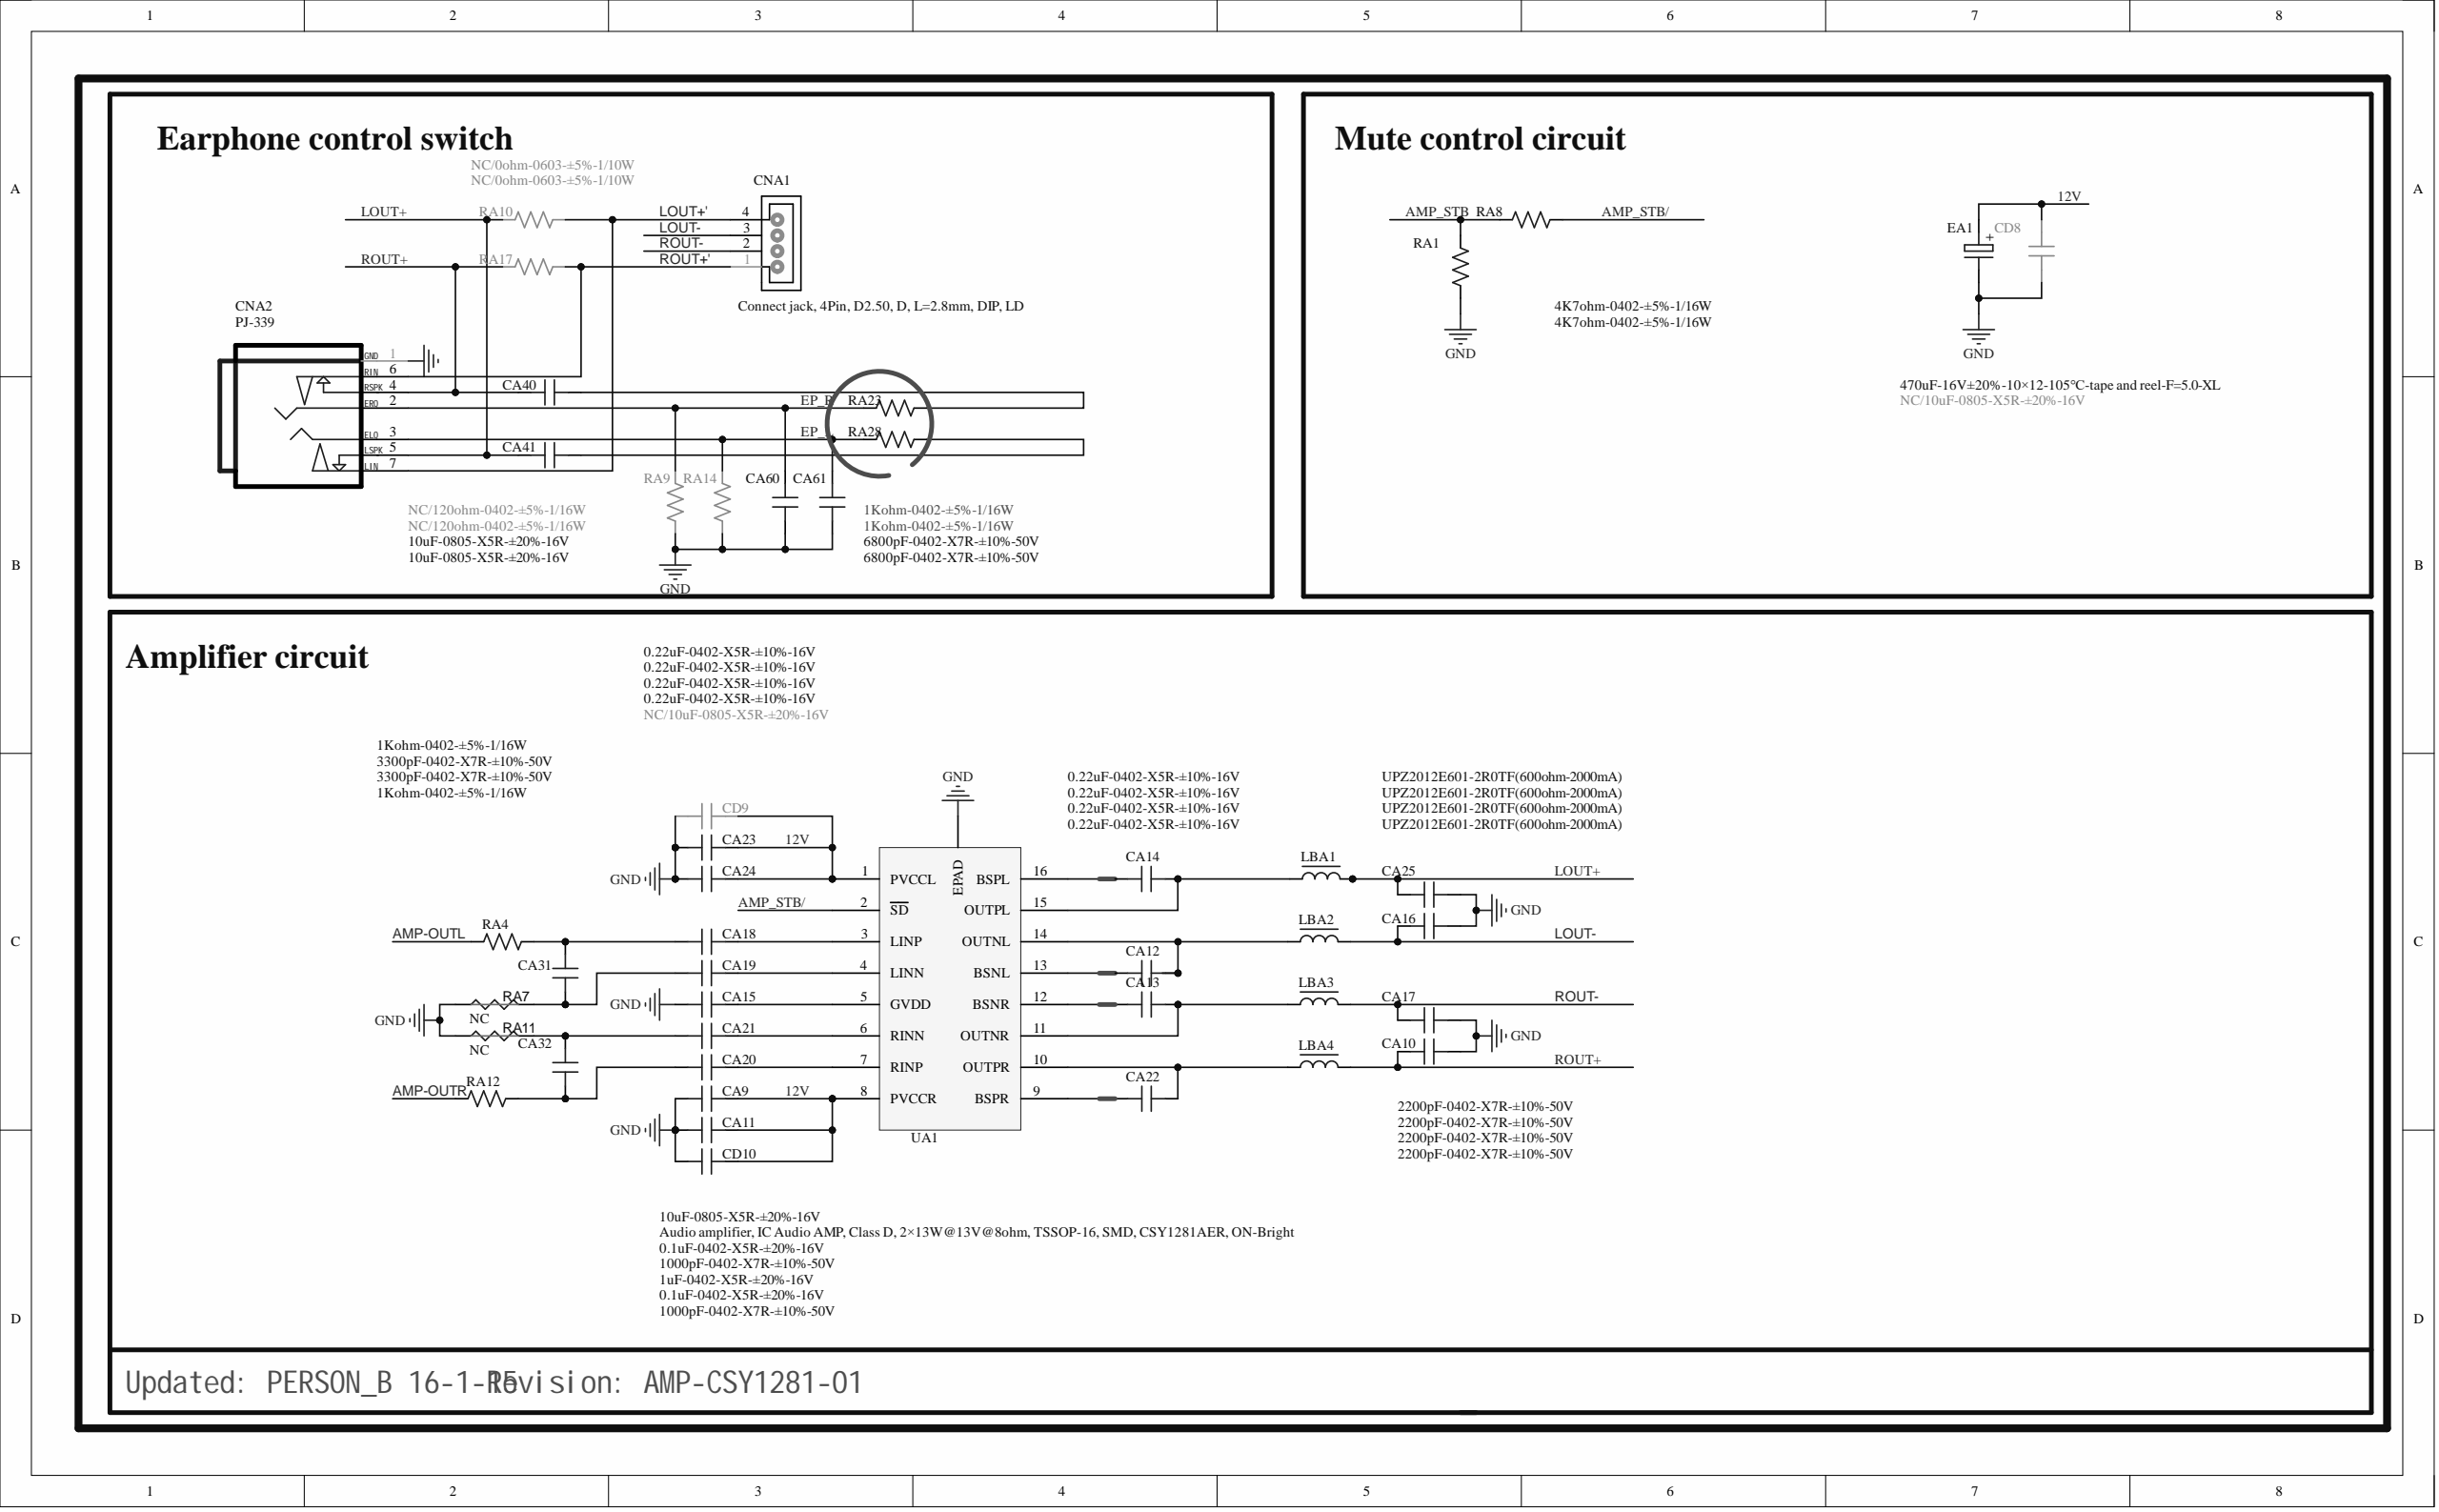Circuit board | Altium Designer | 709 parts | 378 nets | one sheet of the schematic
Parts on this sheet (reference | value | footprint):
CA9 | 1000pF-0402-X7R-±10%-50V | C0402
CA10 | 2200pF-0402-X7R-±10%-50V | C0402
CA11 | 0.1uF-0402-X5R-±20%-16V | C0402
CA12 | 0.22uF-0402-X5R-±10%-16V | C0402
CA13 | 0.22uF-0402-X5R-±10%-16V | C0402
CA14 | 0.22uF-0402-X5R-±10%-16V | C0402
CA15 | 1uF-0402-X5R-±20%-16V | C0402
CA16 | 2200pF-0402-X7R-±10%-50V | C0402
CA17 | 2200pF-0402-X7R-±10%-50V | C0402
CA18 | 0.22uF-0402-X5R-±10%-16V | C0402
CA19 | 0.22uF-0402-X5R-±10%-16V | C0402
CA20 | 0.22uF-0402-X5R-±10%-16V | C0402
CA21 | 0.22uF-0402-X5R-±10%-16V | C0402
CA22 | 0.22uF-0402-X5R-±10%-16V | C0402
CA23 | 0.1uF-0402-X5R-±20%-16V | C0402
CA24 | 1000pF-0402-X7R-±10%-50V | C0402
CA25 | 2200pF-0402-X7R-±10%-50V | C0402
CA31 | 3300pF-0402-X7R-±10%-50V | C0402
CA32 | 3300pF-0402-X7R-±10%-50V | C0402
CA40 | 10uF-0805-X5R-±20%-16V | C0805
CA41 | 10uF-0805-X5R-±20%-16V | C0805
CA60 | 6800pF-0402-X7R-±10%-50V | C0402
CD8 | NC/10uF-0805-X5R-±20%-16V | C0805
CD9 | NC/10uF-0805-X5R-±20%-16V | C0805
CD10 | 10uF-0805-X5R-±20%-16V | C0805
CNA1 | Connect jack, 4Pin, D2.50, D, L=2.8mm, DIP, LD | SIP4/2.54D-1
CNA2 | PJ-339 | PHONE-HD-12
EA1 | 470uF-16V±20%-10×12-105℃-tape and reel-F=5.0-XL | EC(10*12)-V-5
LBA1 | UPZ2012E601-2R0TF(600ohm-2000mA) | L0805
LBA2 | UPZ2012E601-2R0TF(600ohm-2000mA) | L0805
LBA3 | UPZ2012E601-2R0TF(600ohm-2000mA) | L0805
LBA4 | UPZ2012E601-2R0TF(600ohm-2000mA) | L0805
RA1 | 4K7ohm-0402-±5%-1/16W | R0402
RA4 | 1Kohm-0402-±5%-1/16W | R0402
RA7 | NC | GND
RA8 | 4K7ohm-0402-±5%-1/16W | R0402
RA9 | NC/120ohm-0402-±5%-1/16W | R0402
RA10 | NC/0ohm-0603-±5%-1/10W | R0603
RA11 | NC | GND
RA12 | 1Kohm-0402-±5%-1/16W | R0402
RA14 | NC/120ohm-0402-±5%-1/16W | R0402
RA17 | NC/0ohm-0603-±5%-1/10W | R0603
RA23 | 1Kohm-0402-±5%-1/16W | R0402
RA28 | 1Kohm-0402-±5%-1/16W | R0402
UA1 | Audio amplifier, IC Audio AMP, Class D, 2×13W@13V@8ohm, TSSOP-16, SMD, CSY1281AER, ON-Bright | SOP16/1.27-7
Nets of these parts (net: part-pin ...):
ROUT-: CA17-1 CNA1-2 LBA3-2
ROUT+': CNA1-1 CNA2-6 RA17-2
ROUT+: CA10-1 CA40-2 CNA2-4 LBA4-2 RA17-1
NetCA41_1: CA41-1 RA28-2
NetCA40_1: CA40-1 RA23-2
NetCA22_2: CA22-2 LBA4-1 UA1-10
NetCA22_1: CA22-1 UA1-9
NetCA21_2: CA21-2 CA32-2 RA11-JP_1K
NetCA21_1: CA21-1 UA1-6
NetCA20_2: CA20-2 CA32-1 RA12-2
NetCA20_1: CA20-1 UA1-7
NetCA19_2: CA19-2 CA31-1 RA7-JP_1K
NetCA19_1: CA19-1 UA1-4
NetCA18_2: CA18-2 CA31-2 RA4-2
NetCA18_1: CA18-1 UA1-3
NetCA15_2: CA15-2 UA1-5
NetCA14_2: CA14-2 LBA1-1 UA1-15
NetCA14_1: CA14-1 UA1-16
NetCA13_2: CA13-2 LBA3-1 UA1-11
NetCA13_1: CA13-1 UA1-12
NetCA12_2: CA12-2 LBA2-1 UA1-14
NetCA12_1: CA12-1 UA1-13
LOUT-: CA16-2 CNA1-3 LBA2-2
LOUT+': CNA1-4 CNA2-7 RA10-2
LOUT+: CA25-1 CA41-2 CNA2-5 LBA1-2 RA10-1
GND: CA9-2 CA10-2 CA11-2 CA15-1 CA16-1 CA17-2 CA23-2 CA24-2 CA25-2 CA60-2 CD8-2 CD9-1 CD10-1 CNA2-1 EA1-2 RA1-1 RA7-JP_2K RA9-1 RA11-JP_2K RA14-1 UA1-EPAD
EP_R: CA60-1 CNA2-2 RA9-2 RA23-1
EP_L: CNA2-3 RA14-2 RA28-1
AMP_STB/: RA8-2 UA1-2
AMP_STB: RA1-2 RA8-1
AMP-OUTR: RA12-1
AMP-OUTL: RA4-1
12V: CA9-1 CA11-1 CA23-1 CA24-1 CD8-1 CD9-2 CD10-2 EA1-1 UA1-1 UA1-8